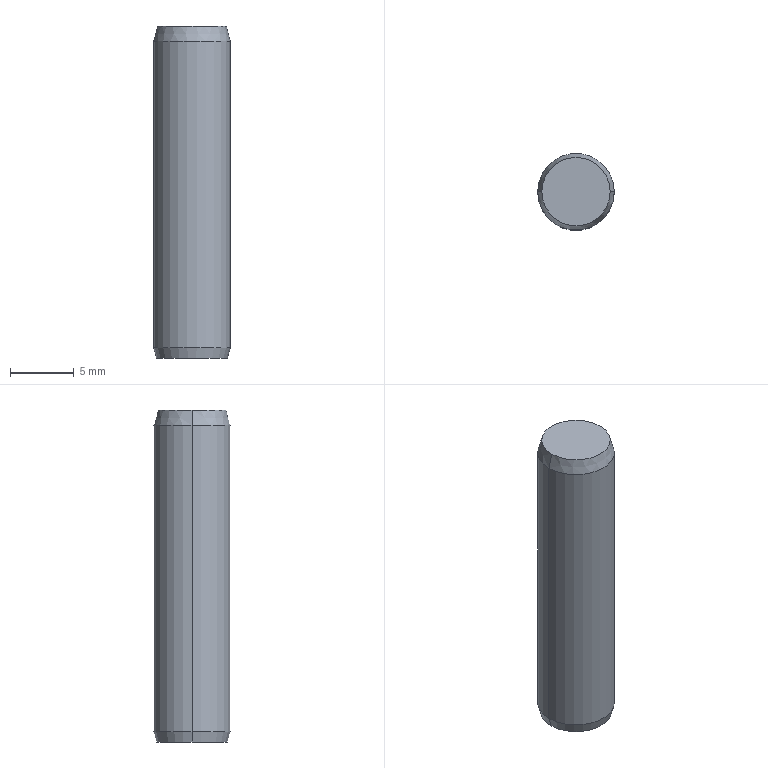Part | SolidWorks | features Chamfer 3, Cut 2, Extrusion 1, RevCut 1 | 1 solid | 16 faces | box 6 x 6 x 26 mm | volume 626.54 mm3 | cone 8 | cylinder 6 | plane 2 | commonest cylinder face diameters 3.464 x2 4.3 x2 6 x2
STEP:
#1=CARTESIAN_POINT('',(1.732,0.,1.418));
#2=VERTEX_POINT('',#1);
#3=CARTESIAN_POINT('',(-1.732,0.,1.418));
#4=VERTEX_POINT('',#3);
#5=CARTESIAN_POINT('',(0.,0.,1.418));
#6=DIRECTION('',(0.,0.,-1.));
#7=DIRECTION('',(-1.,0.,0.));
#8=AXIS2_PLACEMENT_3D('',#5,#6,#7);
#9=CIRCLE('',#8,1.732);
#10=EDGE_CURVE('',#2,#4,#9,.T.);
#11=ORIENTED_EDGE('',*,*,#10,.F.);
#12=CARTESIAN_POINT('',(2.15,0.,1.));
#13=VERTEX_POINT('',#12);
#14=CARTESIAN_POINT('',(2.15,0.,1.));
#15=DIRECTION('',(0.7071,0.,-0.7071));
#16=VECTOR('',#15,1000.);
#17=LINE('',#14,#16);
#18=EDGE_CURVE('',#2,#13,#17,.T.);
#19=ORIENTED_EDGE('',*,*,#18,.T.);
#20=CARTESIAN_POINT('',(-2.15,0.,1.));
#21=VERTEX_POINT('',#20);
#22=CARTESIAN_POINT('',(0.,0.,1.));
#23=DIRECTION('',(0.,0.,-1.));
#24=DIRECTION('',(-1.,0.,0.));
#25=AXIS2_PLACEMENT_3D('',#22,#23,#24);
#26=CIRCLE('',#25,2.15);
#27=EDGE_CURVE('',#13,#21,#26,.T.);
#28=ORIENTED_EDGE('',*,*,#27,.T.);
#29=CARTESIAN_POINT('',(-2.15,0.,1.));
#30=DIRECTION('',(-0.7071,0.,-0.7071));
#31=VECTOR('',#30,1000.);
#32=LINE('',#29,#31);
#33=EDGE_CURVE('',#4,#21,#32,.T.);
#34=ORIENTED_EDGE('',*,*,#33,.F.);
#35=EDGE_LOOP('',(#11,#19,#28,#34));
#36=FACE_OUTER_BOUND('',#35,.T.);
#37=CARTESIAN_POINT('',(0.,0.,1.));
#38=DIRECTION('',(0.,0.,-1.));
#39=DIRECTION('',(-1.,0.,0.));
#40=AXIS2_PLACEMENT_3D('',#37,#38,#39);
#41=CONICAL_SURFACE('',#40,2.15,0.7854);
#42=ADVANCED_FACE('',(#36),#41,.F.);
#43=CARTESIAN_POINT('',(-1.732,0.,10.));
#44=VERTEX_POINT('',#43);
#45=CARTESIAN_POINT('',(1.732,0.,10.));
#46=VERTEX_POINT('',#45);
#47=CARTESIAN_POINT('',(0.,0.,10.));
#48=DIRECTION('',(0.,0.,1.));
#49=DIRECTION('',(1.,0.,0.));
#50=AXIS2_PLACEMENT_3D('',#47,#48,#49);
#51=CIRCLE('',#50,1.732);
#52=EDGE_CURVE('',#44,#46,#51,.T.);
#53=ORIENTED_EDGE('',*,*,#52,.T.);
#54=CARTESIAN_POINT('',(1.732,0.,10.));
#55=DIRECTION('',(0.,0.,-1.));
#56=VECTOR('',#55,1000.);
#57=LINE('',#54,#56);
#58=EDGE_CURVE('',#46,#2,#57,.T.);
#59=ORIENTED_EDGE('',*,*,#58,.T.);
#60=ORIENTED_EDGE('',*,*,#10,.T.);
#61=CARTESIAN_POINT('',(-1.732,0.,10.));
#62=DIRECTION('',(0.,0.,-1.));
#63=VECTOR('',#62,1000.);
#64=LINE('',#61,#63);
#65=EDGE_CURVE('',#44,#4,#64,.T.);
#66=ORIENTED_EDGE('',*,*,#65,.F.);
#67=EDGE_LOOP('',(#53,#59,#60,#66));
#68=FACE_OUTER_BOUND('',#67,.T.);
#69=CARTESIAN_POINT('',(0.,0.,10.));
#70=DIRECTION('',(0.,0.,-1.));
#71=DIRECTION('',(-1.,0.,0.));
#72=AXIS2_PLACEMENT_3D('',#69,#70,#71);
#73=CYLINDRICAL_SURFACE('',#72,1.732);
#74=ADVANCED_FACE('',(#68),#73,.F.);
#75=CARTESIAN_POINT('',(0.,0.,11.));
#76=VERTEX_POINT('',#75);
#77=CARTESIAN_POINT('',(-1.732,0.,10.));
#78=DIRECTION('',(-0.866,0.,-0.5));
#79=VECTOR('',#78,1000.);
#80=LINE('',#77,#79);
#81=EDGE_CURVE('',#76,#44,#80,.T.);
#82=ORIENTED_EDGE('',*,*,#81,.F.);
#83=CARTESIAN_POINT('',(1.732,0.,10.));
#84=DIRECTION('',(0.866,0.,-0.5));
#85=VECTOR('',#84,1000.);
#86=LINE('',#83,#85);
#87=EDGE_CURVE('',#76,#46,#86,.T.);
#88=ORIENTED_EDGE('',*,*,#87,.T.);
#89=ORIENTED_EDGE('',*,*,#52,.F.);
#90=EDGE_LOOP('',(#82,#88,#89));
#91=FACE_OUTER_BOUND('',#90,.T.);
#92=CARTESIAN_POINT('',(0.,0.,10.));
#93=DIRECTION('',(0.,0.,-1.));
#94=DIRECTION('',(-1.,0.,0.));
#95=AXIS2_PLACEMENT_3D('',#92,#93,#94);
#96=CONICAL_SURFACE('',#95,1.732,1.047);
#97=ADVANCED_FACE('',(#91),#96,.F.);
#98=ORIENTED_EDGE('',*,*,#27,.F.);
#99=CARTESIAN_POINT('',(2.15,0.,0.));
#100=VERTEX_POINT('',#99);
#101=CARTESIAN_POINT('',(2.15,0.,1.));
#102=DIRECTION('',(0.,0.,-1.));
#103=VECTOR('',#102,1000.);
#104=LINE('',#101,#103);
#105=EDGE_CURVE('',#13,#100,#104,.T.);
#106=ORIENTED_EDGE('',*,*,#105,.T.);
#107=CARTESIAN_POINT('',(-2.15,0.,0.));
#108=VERTEX_POINT('',#107);
#109=CARTESIAN_POINT('',(0.,0.,0.));
#110=DIRECTION('',(0.,0.,-1.));
#111=DIRECTION('',(-1.,0.,0.));
#112=AXIS2_PLACEMENT_3D('',#109,#110,#111);
#113=CIRCLE('',#112,2.15);
#114=EDGE_CURVE('',#100,#108,#113,.T.);
#115=ORIENTED_EDGE('',*,*,#114,.T.);
#116=CARTESIAN_POINT('',(-2.15,0.,1.));
#117=DIRECTION('',(0.,0.,-1.));
#118=VECTOR('',#117,1000.);
#119=LINE('',#116,#118);
#120=EDGE_CURVE('',#21,#108,#119,.T.);
#121=ORIENTED_EDGE('',*,*,#120,.F.);
#122=EDGE_LOOP('',(#98,#106,#115,#121));
#123=FACE_OUTER_BOUND('',#122,.T.);
#124=CARTESIAN_POINT('',(0.,0.,1.));
#125=DIRECTION('',(0.,0.,-1.));
#126=DIRECTION('',(-1.,0.,0.));
#127=AXIS2_PLACEMENT_3D('',#124,#125,#126);
#128=CYLINDRICAL_SURFACE('',#127,2.15);
#129=ADVANCED_FACE('',(#123),#128,.F.);
#130=CARTESIAN_POINT('',(-2.786,0.,0.));
#131=VERTEX_POINT('',#130);
#132=CARTESIAN_POINT('',(2.786,0.,0.));
#133=VERTEX_POINT('',#132);
#134=CARTESIAN_POINT('',(0.,0.,0.));
#135=DIRECTION('',(0.,0.,-1.));
#136=DIRECTION('',(1.,0.,0.));
#137=AXIS2_PLACEMENT_3D('',#134,#135,#136);
#138=CIRCLE('',#137,2.786);
#139=EDGE_CURVE('',#131,#133,#138,.T.);
#140=ORIENTED_EDGE('',*,*,#139,.F.);
#141=CARTESIAN_POINT('',(-3.,0.,0.8));
#142=VERTEX_POINT('',#141);
#143=CARTESIAN_POINT('',(-3.,0.,0.8));
#144=DIRECTION('',(-0.2588,0.,0.9659));
#145=VECTOR('',#144,1000.);
#146=LINE('',#143,#145);
#147=EDGE_CURVE('',#131,#142,#146,.T.);
#148=ORIENTED_EDGE('',*,*,#147,.T.);
#149=CARTESIAN_POINT('',(3.,0.,0.8));
#150=VERTEX_POINT('',#149);
#151=CARTESIAN_POINT('',(0.,0.,0.8));
#152=DIRECTION('',(0.,0.,1.));
#153=DIRECTION('',(1.,0.,0.));
#154=AXIS2_PLACEMENT_3D('',#151,#152,#153);
#155=CIRCLE('',#154,3.);
#156=EDGE_CURVE('',#150,#142,#155,.T.);
#157=ORIENTED_EDGE('',*,*,#156,.F.);
#158=CARTESIAN_POINT('',(3.,0.,0.8));
#159=DIRECTION('',(0.2588,0.,0.9659));
#160=VECTOR('',#159,1000.);
#161=LINE('',#158,#160);
#162=EDGE_CURVE('',#133,#150,#161,.T.);
#163=ORIENTED_EDGE('',*,*,#162,.F.);
#164=EDGE_LOOP('',(#140,#148,#157,#163));
#165=FACE_OUTER_BOUND('',#164,.T.);
#166=CARTESIAN_POINT('',(0.,0.,0.8));
#167=DIRECTION('',(0.,0.,1.));
#168=DIRECTION('',(1.,0.,0.));
#169=AXIS2_PLACEMENT_3D('',#166,#167,#168);
#170=CONICAL_SURFACE('',#169,3.,0.2618);
#171=ADVANCED_FACE('',(#165),#170,.T.);
#172=CARTESIAN_POINT('',(2.678,0.,26.));
#173=VERTEX_POINT('',#172);
#174=CARTESIAN_POINT('',(-2.678,0.,26.));
#175=VERTEX_POINT('',#174);
#176=CARTESIAN_POINT('',(0.,0.,26.));
#177=DIRECTION('',(0.,0.,1.));
#178=DIRECTION('',(1.,0.,0.));
#179=AXIS2_PLACEMENT_3D('',#176,#177,#178);
#180=CIRCLE('',#179,2.678);
#181=EDGE_CURVE('',#173,#175,#180,.T.);
#182=ORIENTED_EDGE('',*,*,#181,.F.);
#183=CARTESIAN_POINT('',(3.,0.,24.8));
#184=VERTEX_POINT('',#183);
#185=CARTESIAN_POINT('',(2.678,0.,26.));
#186=DIRECTION('',(0.2588,0.,-0.9659));
#187=VECTOR('',#186,1000.);
#188=LINE('',#185,#187);
#189=EDGE_CURVE('',#173,#184,#188,.T.);
#190=ORIENTED_EDGE('',*,*,#189,.T.);
#191=CARTESIAN_POINT('',(-3.,0.,24.8));
#192=VERTEX_POINT('',#191);
#193=CARTESIAN_POINT('',(0.,0.,24.8));
#194=DIRECTION('',(0.,0.,-1.));
#195=DIRECTION('',(1.,0.,0.));
#196=AXIS2_PLACEMENT_3D('',#193,#194,#195);
#197=CIRCLE('',#196,3.);
#198=EDGE_CURVE('',#192,#184,#197,.T.);
#199=ORIENTED_EDGE('',*,*,#198,.F.);
#200=CARTESIAN_POINT('',(-2.678,0.,26.));
#201=DIRECTION('',(-0.2588,0.,-0.9659));
#202=VECTOR('',#201,1000.);
#203=LINE('',#200,#202);
#204=EDGE_CURVE('',#175,#192,#203,.T.);
#205=ORIENTED_EDGE('',*,*,#204,.F.);
#206=EDGE_LOOP('',(#182,#190,#199,#205));
#207=FACE_OUTER_BOUND('',#206,.T.);
#208=CARTESIAN_POINT('',(0.,0.,26.));
#209=DIRECTION('',(0.,0.,-1.));
#210=DIRECTION('',(-1.,0.,0.));
#211=AXIS2_PLACEMENT_3D('',#208,#209,#210);
#212=CONICAL_SURFACE('',#211,2.678,0.2618);
#213=ADVANCED_FACE('',(#207),#212,.T.);
#214=ORIENTED_EDGE('',*,*,#198,.T.);
#215=CARTESIAN_POINT('',(3.,0.,26.));
#216=DIRECTION('',(0.,0.,-1.));
#217=VECTOR('',#216,1000.);
#218=LINE('',#215,#217);
#219=EDGE_CURVE('',#184,#150,#218,.T.);
#220=ORIENTED_EDGE('',*,*,#219,.T.);
#221=ORIENTED_EDGE('',*,*,#156,.T.);
#222=CARTESIAN_POINT('',(-3.,0.,26.));
#223=DIRECTION('',(0.,0.,-1.));
#224=VECTOR('',#223,1000.);
#225=LINE('',#222,#224);
#226=EDGE_CURVE('',#192,#142,#225,.T.);
#227=ORIENTED_EDGE('',*,*,#226,.F.);
#228=EDGE_LOOP('',(#214,#220,#221,#227));
#229=FACE_OUTER_BOUND('',#228,.T.);
#230=CARTESIAN_POINT('',(0.,0.,26.));
#231=DIRECTION('',(0.,0.,-1.));
#232=DIRECTION('',(-1.,0.,0.));
#233=AXIS2_PLACEMENT_3D('',#230,#231,#232);
#234=CYLINDRICAL_SURFACE('',#233,3.);
#235=ADVANCED_FACE('',(#229),#234,.T.);
#236=ORIENTED_EDGE('',*,*,#219,.F.);
#237=CARTESIAN_POINT('',(0.,0.,24.8));
#238=DIRECTION('',(0.,0.,-1.));
#239=DIRECTION('',(1.,0.,0.));
#240=AXIS2_PLACEMENT_3D('',#237,#238,#239);
#241=CIRCLE('',#240,3.);
#242=EDGE_CURVE('',#184,#192,#241,.T.);
#243=ORIENTED_EDGE('',*,*,#242,.T.);
#244=ORIENTED_EDGE('',*,*,#226,.T.);
#245=CARTESIAN_POINT('',(0.,0.,0.8));
#246=DIRECTION('',(0.,0.,1.));
#247=DIRECTION('',(1.,0.,0.));
#248=AXIS2_PLACEMENT_3D('',#245,#246,#247);
#249=CIRCLE('',#248,3.);
#250=EDGE_CURVE('',#142,#150,#249,.T.);
#251=ORIENTED_EDGE('',*,*,#250,.T.);
#252=EDGE_LOOP('',(#236,#243,#244,#251));
#253=FACE_OUTER_BOUND('',#252,.T.);
#254=CARTESIAN_POINT('',(0.,0.,26.));
#255=DIRECTION('',(0.,0.,-1.));
#256=DIRECTION('',(-1.,0.,0.));
#257=AXIS2_PLACEMENT_3D('',#254,#255,#256);
#258=CYLINDRICAL_SURFACE('',#257,3.);
#259=ADVANCED_FACE('',(#253),#258,.T.);
#260=CARTESIAN_POINT('',(0.,0.,26.));
#261=DIRECTION('',(0.,0.,1.));
#262=DIRECTION('',(1.,0.,0.));
#263=AXIS2_PLACEMENT_3D('',#260,#261,#262);
#264=CIRCLE('',#263,2.678);
#265=EDGE_CURVE('',#175,#173,#264,.T.);
#266=ORIENTED_EDGE('',*,*,#265,.T.);
#267=ORIENTED_EDGE('',*,*,#181,.T.);
#268=EDGE_LOOP('',(#266,#267));
#269=FACE_OUTER_BOUND('',#268,.T.);
#270=CARTESIAN_POINT('',(0.,0.,26.));
#271=DIRECTION('',(0.,0.,1.));
#272=DIRECTION('',(1.,0.,0.));
#273=AXIS2_PLACEMENT_3D('',#270,#271,#272);
#274=PLANE('',#273);
#275=ADVANCED_FACE('',(#269),#274,.T.);
#276=CARTESIAN_POINT('',(0.,0.,0.));
#277=DIRECTION('',(0.,0.,-1.));
#278=DIRECTION('',(-1.,0.,0.));
#279=AXIS2_PLACEMENT_3D('',#276,#277,#278);
#280=CIRCLE('',#279,2.15);
#281=EDGE_CURVE('',#108,#100,#280,.T.);
#282=ORIENTED_EDGE('',*,*,#281,.F.);
#283=ORIENTED_EDGE('',*,*,#114,.F.);
#284=EDGE_LOOP('',(#282,#283));
#285=FACE_BOUND('',#284,.T.);
#286=CARTESIAN_POINT('',(0.,0.,0.));
#287=DIRECTION('',(0.,0.,-1.));
#288=DIRECTION('',(1.,0.,0.));
#289=AXIS2_PLACEMENT_3D('',#286,#287,#288);
#290=CIRCLE('',#289,2.786);
#291=EDGE_CURVE('',#133,#131,#290,.T.);
#292=ORIENTED_EDGE('',*,*,#291,.T.);
#293=ORIENTED_EDGE('',*,*,#139,.T.);
#294=EDGE_LOOP('',(#292,#293));
#295=FACE_OUTER_BOUND('',#294,.T.);
#296=CARTESIAN_POINT('',(0.,0.,0.));
#297=DIRECTION('',(0.,0.,1.));
#298=DIRECTION('',(1.,0.,0.));
#299=AXIS2_PLACEMENT_3D('',#296,#297,#298);
#300=PLANE('',#299);
#301=ADVANCED_FACE('',(#285,#295),#300,.F.);
#302=ORIENTED_EDGE('',*,*,#189,.F.);
#303=ORIENTED_EDGE('',*,*,#265,.F.);
#304=ORIENTED_EDGE('',*,*,#204,.T.);
#305=ORIENTED_EDGE('',*,*,#242,.F.);
#306=EDGE_LOOP('',(#302,#303,#304,#305));
#307=FACE_OUTER_BOUND('',#306,.T.);
#308=CARTESIAN_POINT('',(0.,0.,26.));
#309=DIRECTION('',(0.,0.,-1.));
#310=DIRECTION('',(-1.,0.,0.));
#311=AXIS2_PLACEMENT_3D('',#308,#309,#310);
#312=CONICAL_SURFACE('',#311,2.678,0.2618);
#313=ADVANCED_FACE('',(#307),#312,.T.);
#314=ORIENTED_EDGE('',*,*,#147,.F.);
#315=ORIENTED_EDGE('',*,*,#291,.F.);
#316=ORIENTED_EDGE('',*,*,#162,.T.);
#317=ORIENTED_EDGE('',*,*,#250,.F.);
#318=EDGE_LOOP('',(#314,#315,#316,#317));
#319=FACE_OUTER_BOUND('',#318,.T.);
#320=CARTESIAN_POINT('',(0.,0.,0.8));
#321=DIRECTION('',(0.,0.,1.));
#322=DIRECTION('',(1.,0.,0.));
#323=AXIS2_PLACEMENT_3D('',#320,#321,#322);
#324=CONICAL_SURFACE('',#323,3.,0.2618);
#325=ADVANCED_FACE('',(#319),#324,.T.);
#326=ORIENTED_EDGE('',*,*,#105,.F.);
#327=CARTESIAN_POINT('',(0.,0.,1.));
#328=DIRECTION('',(0.,0.,-1.));
#329=DIRECTION('',(-1.,0.,0.));
#330=AXIS2_PLACEMENT_3D('',#327,#328,#329);
#331=CIRCLE('',#330,2.15);
#332=EDGE_CURVE('',#21,#13,#331,.T.);
#333=ORIENTED_EDGE('',*,*,#332,.F.);
#334=ORIENTED_EDGE('',*,*,#120,.T.);
#335=ORIENTED_EDGE('',*,*,#281,.T.);
#336=EDGE_LOOP('',(#326,#333,#334,#335));
#337=FACE_OUTER_BOUND('',#336,.T.);
#338=CARTESIAN_POINT('',(0.,0.,1.));
#339=DIRECTION('',(0.,0.,-1.));
#340=DIRECTION('',(-1.,0.,0.));
#341=AXIS2_PLACEMENT_3D('',#338,#339,#340);
#342=CYLINDRICAL_SURFACE('',#341,2.15);
#343=ADVANCED_FACE('',(#337),#342,.F.);
#344=ORIENTED_EDGE('',*,*,#87,.F.);
#345=ORIENTED_EDGE('',*,*,#81,.T.);
#346=CARTESIAN_POINT('',(0.,0.,10.));
#347=DIRECTION('',(0.,0.,1.));
#348=DIRECTION('',(1.,0.,0.));
#349=AXIS2_PLACEMENT_3D('',#346,#347,#348);
#350=CIRCLE('',#349,1.732);
#351=EDGE_CURVE('',#46,#44,#350,.T.);
#352=ORIENTED_EDGE('',*,*,#351,.F.);
#353=EDGE_LOOP('',(#344,#345,#352));
#354=FACE_OUTER_BOUND('',#353,.T.);
#355=CARTESIAN_POINT('',(0.,0.,10.));
#356=DIRECTION('',(0.,0.,-1.));
#357=DIRECTION('',(-1.,0.,0.));
#358=AXIS2_PLACEMENT_3D('',#355,#356,#357);
#359=CONICAL_SURFACE('',#358,1.732,1.047);
#360=ADVANCED_FACE('',(#354),#359,.F.);
#361=ORIENTED_EDGE('',*,*,#58,.F.);
#362=ORIENTED_EDGE('',*,*,#351,.T.);
#363=ORIENTED_EDGE('',*,*,#65,.T.);
#364=CARTESIAN_POINT('',(0.,0.,1.418));
#365=DIRECTION('',(0.,0.,-1.));
#366=DIRECTION('',(-1.,0.,0.));
#367=AXIS2_PLACEMENT_3D('',#364,#365,#366);
#368=CIRCLE('',#367,1.732);
#369=EDGE_CURVE('',#4,#2,#368,.T.);
#370=ORIENTED_EDGE('',*,*,#369,.T.);
#371=EDGE_LOOP('',(#361,#362,#363,#370));
#372=FACE_OUTER_BOUND('',#371,.T.);
#373=CARTESIAN_POINT('',(0.,0.,10.));
#374=DIRECTION('',(0.,0.,-1.));
#375=DIRECTION('',(-1.,0.,0.));
#376=AXIS2_PLACEMENT_3D('',#373,#374,#375);
#377=CYLINDRICAL_SURFACE('',#376,1.732);
#378=ADVANCED_FACE('',(#372),#377,.F.);
#379=ORIENTED_EDGE('',*,*,#18,.F.);
#380=ORIENTED_EDGE('',*,*,#369,.F.);
#381=ORIENTED_EDGE('',*,*,#33,.T.);
#382=ORIENTED_EDGE('',*,*,#332,.T.);
#383=EDGE_LOOP('',(#379,#380,#381,#382));
#384=FACE_OUTER_BOUND('',#383,.T.);
#385=CARTESIAN_POINT('',(0.,0.,1.));
#386=DIRECTION('',(0.,0.,-1.));
#387=DIRECTION('',(-1.,0.,0.));
#388=AXIS2_PLACEMENT_3D('',#385,#386,#387);
#389=CONICAL_SURFACE('',#388,2.15,0.7854);
#390=ADVANCED_FACE('',(#384),#389,.F.);
#391=CLOSED_SHELL('',(#42,#74,#97,#129,#171,#213,#235,#259,#275,#301,#313,#325,#343,#360,#378,#390));
#392=MANIFOLD_SOLID_BREP('',#391);
#393=CARTESIAN_POINT('',(0.,0.,0.));
#394=DIRECTION('',(0.,0.,1.));
#395=DIRECTION('',(1.,0.,0.));
#396=AXIS2_PLACEMENT_3D('',#393,#394,#395);
#397=(LENGTH_UNIT()NAMED_UNIT(*)SI_UNIT(.MILLI.,.METRE.));
#398=UNCERTAINTY_MEASURE_WITH_UNIT(LENGTH_MEASURE(0.00001),#397,'','');
#399=(NAMED_UNIT(*)PLANE_ANGLE_UNIT()SI_UNIT($,.RADIAN.));
#400=(NAMED_UNIT(*)SI_UNIT($,.STERADIAN.)SOLID_ANGLE_UNIT());
#401=(GEOMETRIC_REPRESENTATION_CONTEXT(3)GLOBAL_UNCERTAINTY_ASSIGNED_CONTEXT((#398))GLOBAL_UNIT_ASSIGNED_CONTEXT((#397,#399,#400))REPRESENTATION_CONTEXT('',''));
#402=ADVANCED_BREP_SHAPE_REPRESENTATION('',(#392,#396),#401);